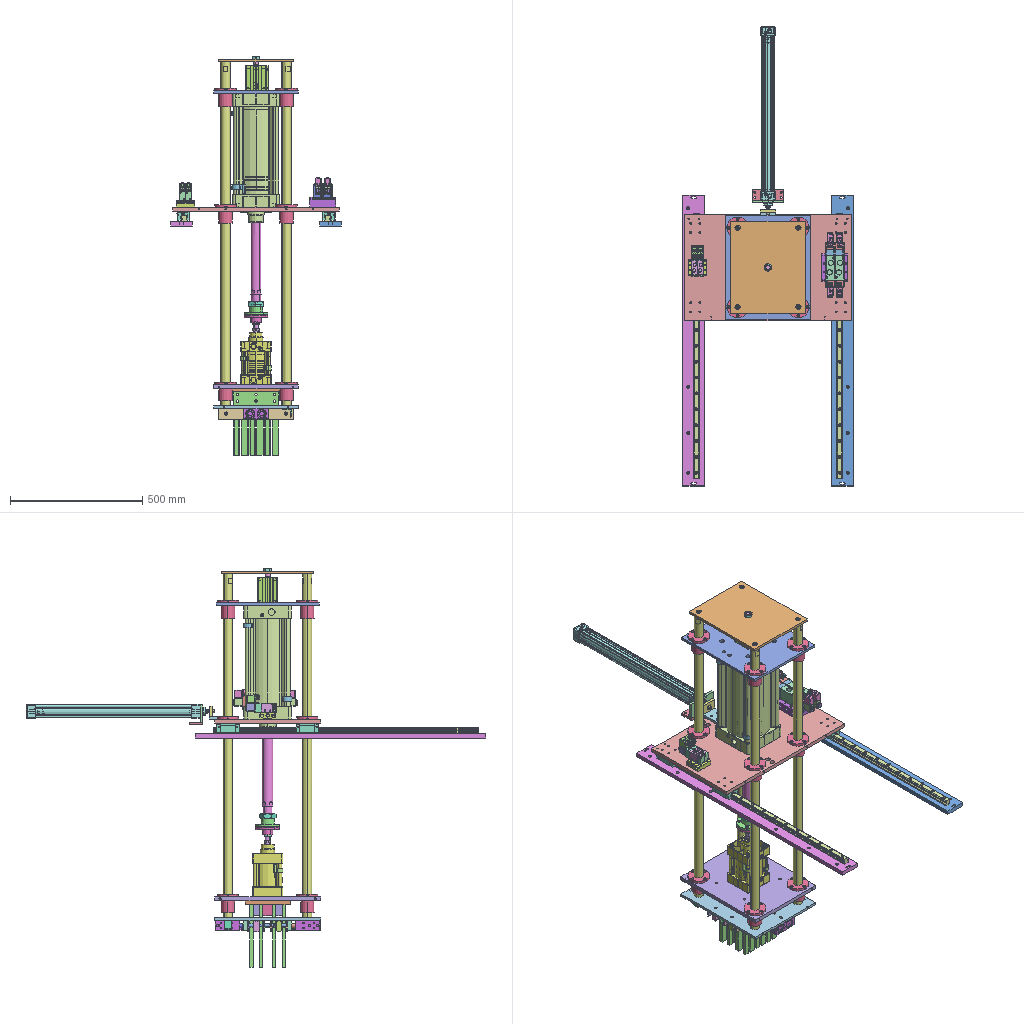Assembly | STEP file | 79 different items | 179 placed | box 643 x 1739 x 1508 mm
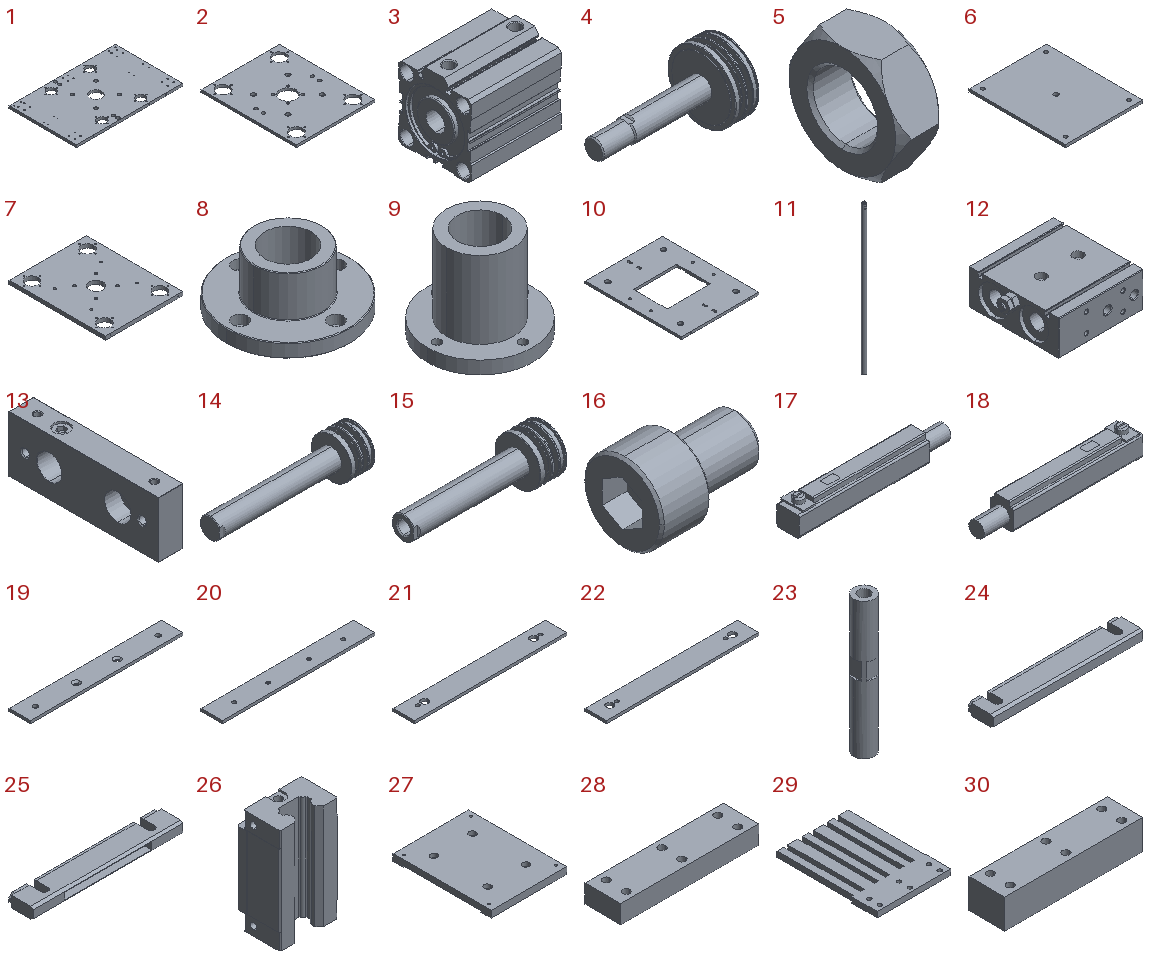Parts list (item | name | quantity | parent item | size | volume):
1 | 44-02-17 Press Cylinder Mounting Plate | x1 | in 44-01-00 Press-fit Slot Insertion Section2 | 630 x 400 x 15 mm | 3544491 mm3
2 | 44-02-18 Locating Cylinder Mounting Plate | x1 | in 44-01-00 Press-fit Slot Insertion Section2 | 320 x 390 x 10 mm | 1104020 mm3
3 | ACQS_63x50-1 | x1 | - | 96 x 77 x 84 mm | 270939 mm3
4 | ACQS_63x50-2 | x1 | - | 122 x 62.5 x 62.5 mm | 85364 mm3
5 | ACQS_63x50-3 | x1 | - | 11 x 31.177 x 27 mm | 4519 mm3
6 | 44-02-04 Locating Push Plate | x1 | in 44-01-00 Press-fit Slot Insertion Section2 | 280 x 350 x 10 mm | 972552 mm3
7 | 44-02-19 Press-fit Push Plate | x1 | in 44-01-00 Press-fit Slot Insertion Section2 | 320 x 400 x 15 mm | 1729546 mm3
8 | 44-02-20 Press Cylinder Connector | x1 | in 44-01-00 Press-fit Slot Insertion Section2 | 90 x 90 x 40 mm | 83101 mm3
9 | LHFRD35 | x12 | in 44-01-00 Press-fit Slot Insertion Section2 | 82 x 82 x 70 mm | 110033 mm3
10 | 44-02-21 Press-fit Locating Plate | x1 | in 44-01-00 Press-fit Slot Insertion Section2 | 320 x 400 x 10 mm | 995471 mm3
11 | 44-02-05 Press-fit Guide Shaft | x4 | in 44-01-00 Press-fit Slot Insertion Section2 | 35 x 35 x 1310 mm | 1250098 mm3
12 | TR_32x10-1 | x2 | - | 106 x 98 x 38 mm | 251208 mm3
13 | TR_32x10-2 | x2 | - | 16 x 96 x 36 mm | 48259 mm3
14 | TR_32x10-3 | x2 | - | 114.8 x 31.6 x 31.6 mm | 30621 mm3
15 | TR_32x10-4 | x2 | - | 98.8 x 31.6 x 31.6 mm | 26490 mm3
16 | TR_32x10-5 | x2 | - | 23.5 x 16 x 16 mm | 2769 mm3
17 | TR_32x10-6 | x2 | - | 30.5 x 4.4 x 5.5 mm | 552.742 mm3
18 | TR_32x10-7 | x2 | - | 30.5 x 4.4 x 5.5 mm | 552.742 mm3
19 | 44-02-06 Ear Forming Push Plate A | x1 | in 44-01-00 Press-fit Slot Insertion Section2 | 280 x 39 x 5 mm | 53413 mm3
20 | 44-02-07 Ear Forming Push Plate B | x1 | in 44-01-00 Press-fit Slot Insertion Section2 | 280 x 39 x 5 mm | 53633 mm3
21 | 44-02-08 Ear Forming Plate A | x1 | in 44-01-00 Press-fit Slot Insertion Section2 | 280 x 39 x 5 mm | 52910 mm3
22 | 44-02-09 Ear Forming Plate B | x1 | in 44-01-00 Press-fit Slot Insertion Section2 | 280 x 39 x 5 mm | 52910 mm3
23 | 44-02-10 Ear Forming Connecting Rod | x4 | in 44-01-00 Press-fit Slot Insertion Section2 | 12 x 12 x 81 mm | 7569 mm3
24 | 44-02-22 Ear Forming Locating Plate B | x1 | in 44-01-00 Press-fit Slot Insertion Section2 | 280 x 46 x 20.7 mm | 241213 mm3
25 | 44-02-23 Ear Forming Locating Plate C | x1 | in 44-01-00 Press-fit Slot Insertion Section2 | 280 x 46 x 20.7 mm | 145134 mm3
26 | HGH25CA | x4 | in 44-01-00 Press-fit Slot Insertion Section2 | 48 x 34.5 x 84 mm | 100839 mm3
27 | 44-02-013 Press-fit Fixing Plate | x1 | in 44-02-012 Press Plate Assembly | 170 x 220 x 15 mm | 464467 mm3
28 | 44-02-14 Press-fit Locating Plate | x2 | in 44-02-012 Press Plate Assembly | 173 x 45 x 23 mm | 168792 mm3
29 | 44-02-15 Press Plate | x4 | in 44-02-012 Press Plate Assembly | 173 x 240 x 13 mm | 402588 mm3
30 | 44-02-16 Press-fit Connecting Plate | x1 | in 44-02-012 Press Plate Assembly | 173 x 45 x 37 mm | 273922 mm3
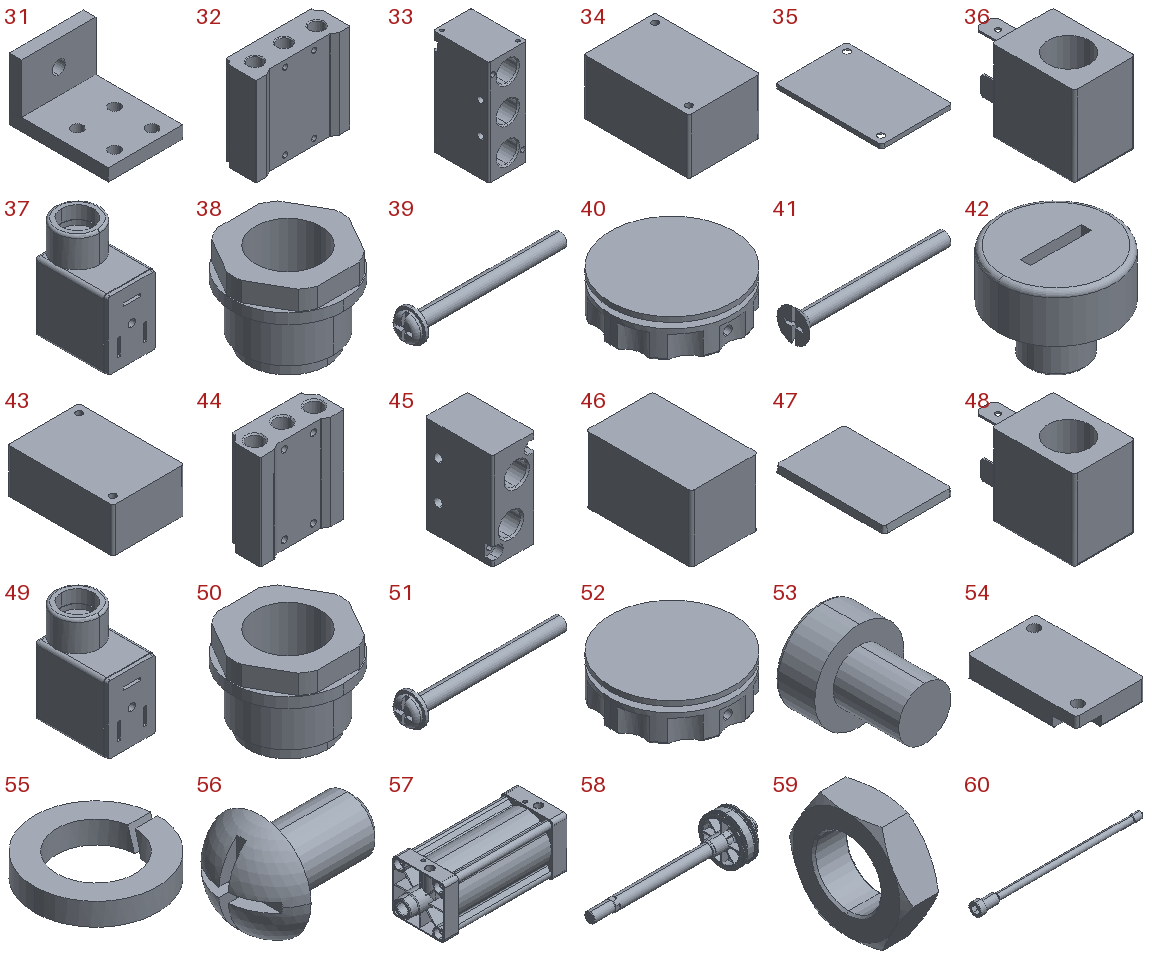31 | 44-02-011 Press Platform Push Plate | x1 | in 44-01-00 Press-fit Slot Insertion Section2 | 60 x 80 x 50 mm | 68539 mm3
32 | 400M_2F_400M-2F | x1 | in 44-01-00 Press-fit Slot Insertion Section2 | 104 x 38 x 98 mm | 289660 mm3
33 | 4V430C_15_Valve_Body | x2 | in 4V430C_15_B_4V430C-15-B | 34 x 50 x 94 mm | 133275 mm3
34 | 4V430C_15_Valve_Switch | x4 | in 4V430C_15_B_4V430C-15-B | 34 x 50 x 26.2 mm | 44112 mm3
35 | 4V430C_15_Valve_Board | x4 | in 4V430C_15_B_4V430C-15-B | 33.2 x 49.5 x 2 mm | 3202 mm3
36 | 4V430C_15_Valve_Coil | x4 | in 4V430C_15_B_4V430C-15-B | 22.3 x 44.2 x 30 mm | 14846 mm3
37 | 4V430C_15_Valve_Terminal | x4 | in 4V430C_15_B_4V430C-15-B | 21 x 32.2 x 41.5 mm | 20201 mm3
38 | 4V430C_15_Valve_Nut_T | x4 | in 4V430C_15_B_4V430C-15-B | 18.4 x 18.4 x 14 mm | 1443 mm3
39 | 4V430C_15_Valve_Bolt | x4 | in 4V430C_15_B_4V430C-15-B | 33.2 x 6.5 x 6.5 mm | 266.857 mm3
40 | 4V430C_15_Valve_Nut_C | x4 | in 4V430C_15_B_4V430C-15-B | 20 x 20 x 6.2 mm | 1695 mm3
41 | 4V430C_15_Valve_Screw_L | x8 | in 4V430C_15_B_4V430C-15-B | 32.2 x 7 x 6.954 mm | 247.49 mm3
42 | 4V430C_15_Valve_Button | x4 | in 4V430C_15_B_4V430C-15-B | 6.8 x 6.8 x 5.6 mm | 124.339 mm3
43 | 4V430C_15_Valve_Cover | x2 | in 4V430C_15_B_4V430C-15-B | 34 x 50 x 21 mm | 35377 mm3
44 | 200M_2F_200M-2F | x1 | in 44-01-00 Press-fit Slot Insertion Section2 | 61 x 26 x 69 mm | 73969 mm3
45 | - | x2 | in 4V210_08_B_4V210-08-B-P | 22 x 35 x 50 mm | 32799 mm3
46 | - | x2 | in 4V210_08_B_4V210-08-B-P | 22 x 35 x 22 mm | 16858 mm3
47 | - | x2 | in 4V210_08_B_4V210-08-B-P | 22 x 35 x 2.2 mm | 1664 mm3
48 | 4V200_Coil | x2 | in 4V210_08_B_4V210-08-B-P | 22.3 x 44.2 x 30 mm | 14846 mm3
49 | 4V200_Terminal | x2 | in 4V210_08_B_4V210-08-B-P | 21 x 32.2 x 41.5 mm | 20201 mm3
50 | 4V200_Terminal_Nut | x2 | in 4V210_08_B_4V210-08-B-P | 18.4 x 18.4 x 14 mm | 1443 mm3
51 | 4V200_Bolt | x2 | in 4V210_08_B_4V210-08-B-P | 33.2 x 6.5 x 6.5 mm | 266.857 mm3
52 | 4V200_Nut_C | x2 | in 4V210_08_B_4V210-08-B-P | 20 x 20 x 6.2 mm | 1695 mm3
53 | - | x2 | in 4V210_08_B_4V210-08-B-P | 6.8 x 8 x 6.8 mm | 164.101 mm3
54 | - | x2 | in 4V210_08_B_4V210-08-B-P | 22 x 35 x 6.7 mm | 4712 mm3
55 | - | x4 | in 4V210_08_B_4V210-08-B-P | 5.5 x 5.5 x 1 mm | 13.826 mm3
56 | - | x4 | in 4V210_08_B_4V210-08-B-P | 6.978 x 5.5 x 5.5 mm | 60.193 mm3
57 | - | x1 | - | 492 x 180 x 180 mm | 3117873 mm3
58 | - | x1 | - | 570 x 159 x 159 mm | 1181996 mm3
59 | - | x1 | - | 18 x 63.509 x 55 mm | 30482 mm3
60 | SI160_250 | x4 | - | 400 x 30 x 30 mm | 76937 mm3
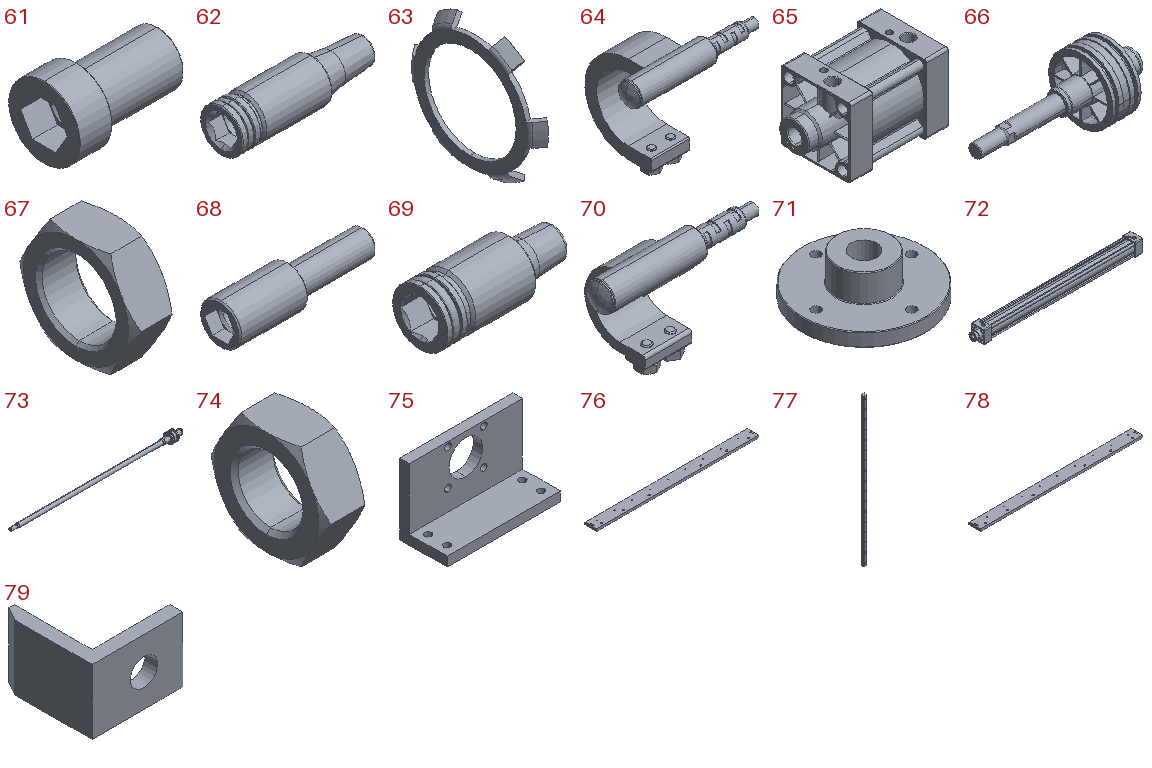61 | SI160 | x4 | - | 48 x 30 x 30 mm | 14480 mm3
62 | 160_C_Screw | x2 | - | 40 x 12 x 12 mm | 3167 mm3
63 | Outer_ring_gear_2 | x2 | - | 1.224 x 12 x 11.247 mm | 16.794 mm3
64 | CS1_B6 | x2 | - | 53.8 x 39.45 x 48.2 mm | 8992 mm3
65 | - | x1 | - | 203 x 115 x 115 mm | 819045 mm3
66 | - | x1 | - | 243 x 99 x 99 mm | 277761 mm3
67 | - | x1 | - | 10 x 30.022 x 26 mm | 3125 mm3
68 | SI100_25 | x8 | - | 55 x 15.5 x 15.5 mm | 5807 mm3
69 | 100_C_Screw | x2 | - | 24.2 x 10 x 10 mm | 1321 mm3
70 | CS1_B4 | x2 | - | 53.8 x 25.85 x 38.4 mm | 5585 mm3
71 | 44-02-24 Press Cylinder Connector | x1 | in 44-01-00 Press-fit Slot Insertion Section2 | 90 x 90 x 30 mm | 79238 mm3
72 | SI_40x550-1 | x1 | - | 679.5 x 53 x 53 mm | 489636 mm3
73 | SI_40x550-2 | x1 | - | 695.5 x 39.5 x 39.5 mm | 154171 mm3
74 | SI_40x550-3 | x1 | - | 7 x 19.63 x 17 mm | 1102 mm3
75 | 44-02-03 Cylinder Mounting Kit | x1 | in 44-01-00 Press-fit Slot Insertion Section2 | 120 x 50 x 75 mm | 124742 mm3
76 | 44-02-01 Guide Rail Mounting Plate A | x1 | in 44-01-00 Press-fit Slot Insertion Section2 | 1100 x 80 x 16 mm | 1395246 mm3
77 | HGH 25HA-950 | x2 | in 44-01-00 Press-fit Slot Insertion Section2 | 23 x 22 x 1000 mm | 420521 mm3
78 | 44-02-02 Guide Rail Mounting Plate B | x1 | in 44-01-00 Press-fit Slot Insertion Section2 | 1100 x 80 x 16 mm | 1395246 mm3
79 | 44-02-25 Lower Ejector Guide Plate | x2 | in 44-01-00 Press-fit Slot Insertion Section2 | 35 x 35 x 25 mm | 7497 mm3
Placements (level | parent | child | x y z in mm | rotation matrix by rows):
1 | 44-01-00 Press-fit Slot Insertion Section2 | 44-02-17 Press Cylinder Mounting Plate | -20.096 -11.932 -0.0 | 1 0 0 0 1 0 0 0 1
1 | 44-01-00 Press-fit Slot Insertion Section2 | 44-02-18 Locating Cylinder Mounting Plate | -20.096 -11.932 437.5 | 1 0 0 0 1 0 0 0 1
1 | 44-01-00 Press-fit Slot Insertion Section2 | subassembly 2 | -20.096 -11.932 543.5 | 0 0 1 0 1 0 -1 0 0
2 | subassembly 2 | ACQS_63x50-1 | -0.0 -0.0 -0.0 | 1 0 0 0 1 0 0 0 1
2 | subassembly 2 | ACQS_63x50-2 | -0.0 -0.0 -0.0 | 1 0 0 0 0.2744 0.9616 0 -0.9616 0.2744
2 | subassembly 2 | ACQS_63x50-3 | -7.5 0.0 -0.0 | 1 0 0 0 0.9981 0.06174 0 -0.06174 0.9981
1 | 44-01-00 Press-fit Slot Insertion Section2 | 44-02-04 Locating Push Plate | -20.096 -11.932 557.5 | -1 0 0 0 -1 0 0 0 1
1 | 44-01-00 Press-fit Slot Insertion Section2 | 44-02-19 Press-fit Push Plate | -20.096 -11.932 -671.0 | 1 0 0 0 1 0 0 0 1
1 | 44-01-00 Press-fit Slot Insertion Section2 | 44-02-20 Press Cylinder Connector | -20.096 -11.932 -399.5 | -0.6148 -0.7887 0 0.7887 -0.6148 0 0 0 1
1 | 44-01-00 Press-fit Slot Insertion Section2 | LHFRD35 | -135.096 138.068 457.5 | -1 0 0 0 1 0 0 0 -1
1 | 44-01-00 Press-fit Slot Insertion Section2 | LHFRD35 | -135.096 -161.932 457.5 | -1 0 0 0 1 0 0 0 -1
1 | 44-01-00 Press-fit Slot Insertion Section2 | LHFRD35 | 94.903 -161.932 457.5 | -1 0 0 0 1 0 0 0 -1
1 | 44-01-00 Press-fit Slot Insertion Section2 | LHFRD35 | 94.903 138.068 457.5 | -1 0 0 0 1 0 0 0 -1
1 | 44-01-00 Press-fit Slot Insertion Section2 | LHFRD35 | 94.903 138.068 17.5 | -1 0 0 0 1 0 0 0 -1
1 | 44-01-00 Press-fit Slot Insertion Section2 | LHFRD35 | 94.903 -161.932 17.5 | -1 0 0 0 1 0 0 0 -1
1 | 44-01-00 Press-fit Slot Insertion Section2 | LHFRD35 | -135.096 138.068 17.5 | -1 0 0 0 1 0 0 0 -1
1 | 44-01-00 Press-fit Slot Insertion Section2 | LHFRD35 | -135.096 -161.932 17.5 | -1 0 0 0 1 0 0 0 -1
1 | 44-01-00 Press-fit Slot Insertion Section2 | LHFRD35 | 94.903 -161.932 -653.5 | -1 0 0 0 1 0 0 0 -1
1 | 44-01-00 Press-fit Slot Insertion Section2 | LHFRD35 | 94.903 138.068 -653.5 | -1 0 0 0 1 0 0 0 -1
1 | 44-01-00 Press-fit Slot Insertion Section2 | LHFRD35 | -135.096 -161.932 -653.5 | -1 0 0 0 1 0 0 0 -1
1 | 44-01-00 Press-fit Slot Insertion Section2 | LHFRD35 | -135.096 138.068 -653.5 | -1 0 0 0 1 0 0 0 -1
1 | 44-01-00 Press-fit Slot Insertion Section2 | 44-02-21 Press-fit Locating Plate | -20.096 -11.932 -748.5 | 1 0 0 0 1 0 0 0 1
1 | 44-01-00 Press-fit Slot Insertion Section2 | 44-02-05 Press-fit Guide Shaft | -135.096 138.068 -88.5 | -0.5385 -0.8426 0 0.8426 -0.5385 0 0 0 1
1 | 44-01-00 Press-fit Slot Insertion Section2 | 44-02-05 Press-fit Guide Shaft | 94.903 138.068 -88.5 | 1 0 0 0 1 0 0 0 1
1 | 44-01-00 Press-fit Slot Insertion Section2 | 44-02-05 Press-fit Guide Shaft | 94.903 -161.932 -88.5 | 0.9008 -0.4343 0 0.4343 0.9008 0 0 0 1
1 | 44-01-00 Press-fit Slot Insertion Section2 | 44-02-05 Press-fit Guide Shaft | -135.096 -161.932 -88.5 | 1 0 0 0 1 0 0 0 1
1 | 44-01-00 Press-fit Slot Insertion Section2 | subassembly 3 | -20.096 -117.932 -753.5 | 0 -1 0 -1 0 0 0 0 -1
2 | subassembly 3 | TR_32x10-1 | -0.0 -0.0 -0.0 | 1 0 0 0 1 0 0 0 1
2 | subassembly 3 | TR_32x10-2 | -0.0 -0.0 -0.0 | 1 0 0 0 1 0 0 0 1
2 | subassembly 3 | TR_32x10-3 | -0.0 -0.0 -0.0 | 1 0 0 0 1 0 0 0 1
2 | subassembly 3 | TR_32x10-4 | -0.0 -0.0 -0.0 | 1 0 0 0 1 0 0 0 1
2 | subassembly 3 | TR_32x10-5 | -0.0 -0.0 -0.0 | 1 0 0 0 1 0 0 0 1
2 | subassembly 3 | TR_32x10-6 | -0.0 -0.0 -0.0 | 1 0 0 0 1 0 0 0 1
2 | subassembly 3 | TR_32x10-7 | -0.0 -0.0 -0.0 | 1 0 0 0 1 0 0 0 1
1 | 44-01-00 Press-fit Slot Insertion Section2 | subassembly 3 | -20.096 94.068 -753.5 | 0 1 0 1 0 0 0 0 -1
2 | subassembly 3 | TR_32x10-1 | -0.0 -0.0 -0.0 | 1 0 0 0 1 0 0 0 1
2 | subassembly 3 | TR_32x10-2 | -0.0 -0.0 -0.0 | 1 0 0 0 1 0 0 0 1
2 | subassembly 3 | TR_32x10-3 | -0.0 -0.0 -0.0 | 1 0 0 0 1 0 0 0 1
2 | subassembly 3 | TR_32x10-4 | -0.0 -0.0 -0.0 | 1 0 0 0 1 0 0 0 1
2 | subassembly 3 | TR_32x10-5 | -0.0 -0.0 -0.0 | 1 0 0 0 1 0 0 0 1
2 | subassembly 3 | TR_32x10-6 | -0.0 -0.0 -0.0 | 1 0 0 0 1 0 0 0 1
2 | subassembly 3 | TR_32x10-7 | -0.0 -0.0 -0.0 | 1 0 0 0 1 0 0 0 1
1 | 44-01-00 Press-fit Slot Insertion Section2 | 44-02-06 Ear Forming Push Plate A | -20.096 -85.432 -772.5 | 1 0 0 0 0 1 0 -1 -0
1 | 44-01-00 Press-fit Slot Insertion Section2 | 44-02-07 Ear Forming Push Plate B | -20.096 61.568 -772.5 | 1 0 0 0 0 1 0 -1 -0
1 | 44-01-00 Press-fit Slot Insertion Section2 | 44-02-08 Ear Forming Plate A | -20.096 0.5677 -772.5 | 1 0 0 0 0 -1 0 1 0
1 | 44-01-00 Press-fit Slot Insertion Section2 | 44-02-09 Ear Forming Plate B | -20.096 -24.432 -772.5 | 1 0 0 0 0 -1 0 1 0
1 | 44-01-00 Press-fit Slot Insertion Section2 | 44-02-10 Ear Forming Connecting Rod | 92.403 -42.432 -772.5 | -0.8372 -0.5469 0 0 0 1 -0.5469 0.8372 -0
1 | 44-01-00 Press-fit Slot Insertion Section2 | 44-02-10 Ear Forming Connecting Rod | -132.596 -42.432 -772.5 | -0.8372 -0.5469 0 0 0 1 -0.5469 0.8372 -0
1 | 44-01-00 Press-fit Slot Insertion Section2 | 44-02-10 Ear Forming Connecting Rod | 79.903 18.568 -772.5 | 1 0 0 0 0 -1 0 1 0
1 | 44-01-00 Press-fit Slot Insertion Section2 | 44-02-10 Ear Forming Connecting Rod | -120.097 18.568 -772.5 | -0.0524 0.9986 0 0 0 -1 -0.9986 -0.0524 0
1 | 44-01-00 Press-fit Slot Insertion Section2 | 44-02-22 Ear Forming Locating Plate B | -20.096 -54.932 -773.5 | 1 0 0 0 0 -1 0 1 0
1 | 44-01-00 Press-fit Slot Insertion Section2 | 44-02-23 Ear Forming Locating Plate C | -20.096 31.068 -773.5 | 1 0 0 0 0 -1 0 1 0
1 | 44-01-00 Press-fit Slot Insertion Section2 | HGH25CA | 254.904 138.068 -47.5 | 1 0 0 0 0 -1 0 1 0
1 | 44-01-00 Press-fit Slot Insertion Section2 | HGH25CA | 254.904 -161.932 -47.5 | 1 0 0 0 0 -1 0 1 0
1 | 44-01-00 Press-fit Slot Insertion Section2 | HGH25CA | -295.096 138.068 -47.5 | 1 0 0 0 0 -1 0 1 0
1 | 44-01-00 Press-fit Slot Insertion Section2 | HGH25CA | -295.096 -161.932 -47.5 | 1 0 0 0 0 -1 0 1 0
1 | 44-01-00 Press-fit Slot Insertion Section2 | 44-02-012 Press Plate Assembly | -47.286 -33.384 -686.0 | 0 1 0 -1 0 0 0 0 1
2 | 44-02-012 Press Plate Assembly | 44-02-013 Press-fit Fixing Plate | -21.452 27.189 -0.0 | 1 0 0 0 1 0 0 0 1
2 | 44-02-012 Press Plate Assembly | 44-02-14 Press-fit Locating Plate | -64.452 27.189 -27.0 | 0 0 1 1 0 0 0 1 0
2 | 44-02-012 Press Plate Assembly | 44-02-14 Press-fit Locating Plate | 21.548 27.189 -27.0 | 0 0 1 1 0 0 0 1 0
2 | 44-02-012 Press Plate Assembly | 44-02-15 Press Plate | -82.452 27.189 -124.5 | 0 0 1 -1 0 0 0 -1 0
2 | 44-02-012 Press Plate Assembly | 44-02-15 Press Plate | -46.452 27.189 -124.5 | 0 0 -1 1 0 0 0 -1 0
2 | 44-02-012 Press Plate Assembly | 44-02-15 Press Plate | 3.548 27.189 -124.5 | 0 0 1 -1 0 0 0 -1 0
2 | 44-02-012 Press Plate Assembly | 44-02-15 Press Plate | 39.548 27.189 -124.5 | 0 0 -1 1 0 0 0 -1 0
2 | 44-02-012 Press Plate Assembly | 44-02-16 Press-fit Connecting Plate | -21.452 27.189 -27.0 | 0 0 -1 -1 0 0 0 1 0
1 | 44-01-00 Press-fit Slot Insertion Section2 | 44-02-011 Press Platform Push Plate | -20.096 168.068 12.5 | 1 0 0 0 1 0 0 0 1
1 | 44-01-00 Press-fit Slot Insertion Section2 | 400M_2F_400M-2F | 183.904 -11.932 7.5 | 0 0 1 1 0 0 0 1 0
1 | 44-01-00 Press-fit Slot Insertion Section2 | 4V430C_15_B_4V430C-15-B | 215.404 -58.932 70.5 | 1 0 0 0 0 -1 0 1 0
2 | 4V430C_15_B_4V430C-15-B | 4V430C_15_Valve_Body | -0.0 -0.0 -0.0 | 1 0 0 0 1 0 0 0 1
2 | 4V430C_15_B_4V430C-15-B | 4V430C_15_Valve_Switch | -0.0 -0.0 -0.0 | -1 0 0 0 1 0 0 0 -1
2 | 4V430C_15_B_4V430C-15-B | 4V430C_15_Valve_Board | -0.0 -0.0 26.2 | -1 0 0 0 1 0 0 0 -1
2 | 4V430C_15_B_4V430C-15-B | 4V430C_15_Valve_Coil | -0.0 -0.0 28.2 | -1 0 0 0 1 0 0 0 -1
2 | 4V430C_15_B_4V430C-15-B | 4V430C_15_Valve_Terminal | -0.0 -0.0 28.2 | -1 0 0 0 1 0 0 0 -1
2 | 4V430C_15_B_4V430C-15-B | 4V430C_15_Valve_Nut_T | -0.0 -0.0 28.2 | -1 0 0 0 1 0 0 0 -1
2 | 4V430C_15_B_4V430C-15-B | 4V430C_15_Valve_Bolt | -0.0 46.7 43.2 | 0 0 1 -1 0 0 0 -1 0
2 | 4V430C_15_B_4V430C-15-B | 4V430C_15_Valve_Nut_C | -0.0 -0.0 28.2 | -1 0 0 0 1 0 0 0 -1
2 | 4V430C_15_B_4V430C-15-B | 4V430C_15_Valve_Screw_L | -13.0 21.0 28.2 | 0 0 1 0 1 0 -1 0 0
2 | 4V430C_15_B_4V430C-15-B | 4V430C_15_Valve_Screw_L | 13.0 -21.0 28.2 | 0 0 1 0 1 0 -1 0 0
2 | 4V430C_15_B_4V430C-15-B | 4V430C_15_Valve_Button | 0.0 25.0 17.6 | -1 0 0 0 0 1 0 1 0
2 | 4V430C_15_B_4V430C-15-B | 4V430C_15_Valve_Cover | -0.0 -0.0 -94.0 | 1 0 0 0 1 0 0 0 1
2 | 4V430C_15_B_4V430C-15-B | 4V430C_15_Valve_Switch | -0.0 -0.0 -115.0 | 1 0 0 0 1 0 0 0 1
2 | 4V430C_15_B_4V430C-15-B | 4V430C_15_Valve_Board | -0.0 -0.0 -141.2 | 1 0 0 0 1 0 0 0 1
2 | 4V430C_15_B_4V430C-15-B | 4V430C_15_Valve_Coil | -0.0 -0.0 -143.2 | 1 0 0 0 1 0 0 0 1
2 | 4V430C_15_B_4V430C-15-B | 4V430C_15_Valve_Terminal | -0.0 -0.0 -143.2 | 1 0 0 0 1 0 0 0 1
2 | 4V430C_15_B_4V430C-15-B | 4V430C_15_Valve_Nut_T | -0.0 -0.0 -143.2 | 1 0 0 0 1 0 0 0 1
2 | 4V430C_15_B_4V430C-15-B | 4V430C_15_Valve_Bolt | -0.0 46.7 -158.2 | 0 0 -1 -1 0 0 0 1 0
2 | 4V430C_15_B_4V430C-15-B | 4V430C_15_Valve_Nut_C | -0.0 -0.0 -143.2 | 1 0 0 0 1 0 0 0 1
2 | 4V430C_15_B_4V430C-15-B | 4V430C_15_Valve_Screw_L | 13.0 21.0 -143.2 | 0 0 -1 0 1 0 1 0 0
2 | 4V430C_15_B_4V430C-15-B | 4V430C_15_Valve_Screw_L | -13.0 -21.0 -143.2 | 0 0 -1 0 1 0 1 0 0
2 | 4V430C_15_B_4V430C-15-B | 4V430C_15_Valve_Button | -0.0 25.0 -132.6 | 1 0 0 0 0 1 0 -1 0
1 | 44-01-00 Press-fit Slot Insertion Section2 | 4V430C_15_B_4V430C-15-B | 250.404 -58.932 70.5 | 1 0 0 0 0 -1 0 1 0
2 | 4V430C_15_B_4V430C-15-B | 4V430C_15_Valve_Body | -0.0 -0.0 -0.0 | 1 0 0 0 1 0 0 0 1
2 | 4V430C_15_B_4V430C-15-B | 4V430C_15_Valve_Switch | -0.0 -0.0 -0.0 | -1 0 0 0 1 0 0 0 -1
2 | 4V430C_15_B_4V430C-15-B | 4V430C_15_Valve_Board | -0.0 -0.0 26.2 | -1 0 0 0 1 0 0 0 -1
2 | 4V430C_15_B_4V430C-15-B | 4V430C_15_Valve_Coil | -0.0 -0.0 28.2 | -1 0 0 0 1 0 0 0 -1
2 | 4V430C_15_B_4V430C-15-B | 4V430C_15_Valve_Terminal | -0.0 -0.0 28.2 | -1 0 0 0 1 0 0 0 -1
2 | 4V430C_15_B_4V430C-15-B | 4V430C_15_Valve_Nut_T | -0.0 -0.0 28.2 | -1 0 0 0 1 0 0 0 -1
2 | 4V430C_15_B_4V430C-15-B | 4V430C_15_Valve_Bolt | -0.0 46.7 43.2 | 0 0 1 -1 0 0 0 -1 0
2 | 4V430C_15_B_4V430C-15-B | 4V430C_15_Valve_Nut_C | -0.0 -0.0 28.2 | -1 0 0 0 1 0 0 0 -1
2 | 4V430C_15_B_4V430C-15-B | 4V430C_15_Valve_Screw_L | -13.0 21.0 28.2 | 0 0 1 0 1 0 -1 0 0
2 | 4V430C_15_B_4V430C-15-B | 4V430C_15_Valve_Screw_L | 13.0 -21.0 28.2 | 0 0 1 0 1 0 -1 0 0
2 | 4V430C_15_B_4V430C-15-B | 4V430C_15_Valve_Button | 0.0 25.0 17.6 | -1 0 0 0 0 1 0 1 0
2 | 4V430C_15_B_4V430C-15-B | 4V430C_15_Valve_Cover | -0.0 -0.0 -94.0 | 1 0 0 0 1 0 0 0 1
2 | 4V430C_15_B_4V430C-15-B | 4V430C_15_Valve_Switch | -0.0 -0.0 -115.0 | 1 0 0 0 1 0 0 0 1
2 | 4V430C_15_B_4V430C-15-B | 4V430C_15_Valve_Board | -0.0 -0.0 -141.2 | 1 0 0 0 1 0 0 0 1
2 | 4V430C_15_B_4V430C-15-B | 4V430C_15_Valve_Coil | -0.0 -0.0 -143.2 | 1 0 0 0 1 0 0 0 1
2 | 4V430C_15_B_4V430C-15-B | 4V430C_15_Valve_Terminal | -0.0 -0.0 -143.2 | 1 0 0 0 1 0 0 0 1
2 | 4V430C_15_B_4V430C-15-B | 4V430C_15_Valve_Nut_T | -0.0 -0.0 -143.2 | 1 0 0 0 1 0 0 0 1
2 | 4V430C_15_B_4V430C-15-B | 4V430C_15_Valve_Bolt | -0.0 46.7 -158.2 | 0 0 -1 -1 0 0 0 1 0
2 | 4V430C_15_B_4V430C-15-B | 4V430C_15_Valve_Nut_C | -0.0 -0.0 -143.2 | 1 0 0 0 1 0 0 0 1
2 | 4V430C_15_B_4V430C-15-B | 4V430C_15_Valve_Screw_L | 13.0 21.0 -143.2 | 0 0 -1 0 1 0 1 0 0
2 | 4V430C_15_B_4V430C-15-B | 4V430C_15_Valve_Screw_L | -13.0 -21.0 -143.2 | 0 0 -1 0 1 0 1 0 0
2 | 4V430C_15_B_4V430C-15-B | 4V430C_15_Valve_Button | -0.0 25.0 -132.6 | 1 0 0 0 0 1 0 -1 0
1 | 44-01-00 Press-fit Slot Insertion Section2 | 200M_2F_200M-2F | -252.096 -11.932 7.5 | 0 0 -1 -1 0 0 0 1 0
1 | 44-01-00 Press-fit Slot Insertion Section2 | 4V210_08_B_4V210-08-B-P | -298.096 -11.932 51.0 | 1 0 0 0 0 -1 0 1 0
2 | 4V210_08_B_4V210-08-B-P | subassembly 4 | -0.0 -0.0 -25.0 | -1 0 0 0 -1 0 0 0 1
2 | 4V210_08_B_4V210-08-B-P | subassembly 5 | -0.0 -0.0 -25.0 | -1 0 0 0 1 0 0 0 -1
2 | 4V210_08_B_4V210-08-B-P | subassembly 6 | -0.0 -0.0 -47.0 | -1 0 0 0 1 0 0 0 -1
2 | 4V210_08_B_4V210-08-B-P | 4V200_Coil | -0.0 -0.0 -49.2 | 1 0 0 0 1 0 0 0 1
2 | 4V210_08_B_4V210-08-B-P | 4V200_Terminal | -0.0 -0.0 -49.2 | 1 0 0 0 1 0 0 0 1
2 | 4V210_08_B_4V210-08-B-P | 4V200_Terminal_Nut | -0.0 -0.0 -49.2 | 1 0 0 0 1 0 0 0 1
2 | 4V210_08_B_4V210-08-B-P | 4V200_Bolt | -0.0 46.7 -64.2 | 0 0 -1 -1 0 0 0 1 0
2 | 4V210_08_B_4V210-08-B-P | 4V200_Nut_C | -0.0 -0.0 -49.2 | 0 1 0 -1 0 0 0 0 1
2 | 4V210_08_B_4V210-08-B-P | subassembly 7 | 0.0 12.5 -38.3 | 0 0 1 0 1 0 -1 0 0
2 | 4V210_08_B_4V210-08-B-P | subassembly 8 | -0.0 -0.0 31.7 | 1 0 0 0 -1 0 0 0 -1
2 | 4V210_08_B_4V210-08-B-P | subassembly 9 | 7.0 -14.0 28.4 | 1 0 0 0 1 0 0 0 1
2 | 4V210_08_B_4V210-08-B-P | subassembly 10 | 7.0 -14.0 29.4 | 0 0 -1 0 -1 0 -1 0 0
2 | 4V210_08_B_4V210-08-B-P | subassembly 9 | -7.0 14.0 28.4 | 1 0 0 0 1 0 0 0 1
2 | 4V210_08_B_4V210-08-B-P | subassembly 10 | -7.0 14.0 29.4 | 0 0 -1 0 -1 0 -1 0 0
1 | 44-01-00 Press-fit Slot Insertion Section2 | 4V210_08_B_4V210-08-B-P | -275.096 -11.932 51.0 | 1 0 0 0 0 -1 0 1 0
2 | 4V210_08_B_4V210-08-B-P | subassembly 4 | -0.0 -0.0 -25.0 | -1 0 0 0 -1 0 0 0 1
2 | 4V210_08_B_4V210-08-B-P | subassembly 5 | -0.0 -0.0 -25.0 | -1 0 0 0 1 0 0 0 -1
2 | 4V210_08_B_4V210-08-B-P | subassembly 6 | -0.0 -0.0 -47.0 | -1 0 0 0 1 0 0 0 -1
2 | 4V210_08_B_4V210-08-B-P | 4V200_Coil | -0.0 -0.0 -49.2 | 1 0 0 0 1 0 0 0 1
2 | 4V210_08_B_4V210-08-B-P | 4V200_Terminal | -0.0 -0.0 -49.2 | 1 0 0 0 1 0 0 0 1
2 | 4V210_08_B_4V210-08-B-P | 4V200_Terminal_Nut | -0.0 -0.0 -49.2 | 1 0 0 0 1 0 0 0 1
2 | 4V210_08_B_4V210-08-B-P | 4V200_Bolt | -0.0 46.7 -64.2 | 0 0 -1 -1 0 0 0 1 0
2 | 4V210_08_B_4V210-08-B-P | 4V200_Nut_C | -0.0 -0.0 -49.2 | 0 1 0 -1 0 0 0 0 1
2 | 4V210_08_B_4V210-08-B-P | subassembly 7 | 0.0 12.5 -38.3 | 0 0 1 0 1 0 -1 0 0
2 | 4V210_08_B_4V210-08-B-P | subassembly 8 | -0.0 -0.0 31.7 | 1 0 0 0 -1 0 0 0 -1
2 | 4V210_08_B_4V210-08-B-P | subassembly 9 | 7.0 -14.0 28.4 | 1 0 0 0 1 0 0 0 1
2 | 4V210_08_B_4V210-08-B-P | subassembly 10 | 7.0 -14.0 29.4 | 0 0 -1 0 -1 0 -1 0 0
2 | 4V210_08_B_4V210-08-B-P | subassembly 9 | -7.0 14.0 28.4 | 1 0 0 0 1 0 0 0 1
2 | 4V210_08_B_4V210-08-B-P | subassembly 10 | -7.0 14.0 29.4 | 0 0 -1 0 -1 0 -1 0 0
1 | 44-01-00 Press-fit Slot Insertion Section2 | subassembly 11 | -20.096 -11.932 7.5 | 0 0 -1 0 1 0 1 0 0
2 | subassembly 11 | subassembly 12 | -0.0 -0.0 -0.0 | 1 0 0 0 1 0 0 0 1
2 | subassembly 11 | subassembly 13 | -250.0 -0.0 -0.0 | 1 0 0 0 0.7071 0.7071 0 -0.7071 0.7071
2 | subassembly 11 | subassembly 14 | -375.0 0.0 0.0 | 1 0 0 0 -1 0 0 0 -1
2 | subassembly 11 | SI160_250 | 50.0 -70.0 70.0 | 1 0 0 0 1 0 0 0 1
2 | subassembly 11 | SI160_250 | 50.0 -70.0 -70.0 | 1 0 0 0 1 0 0 0 1
2 | subassembly 11 | SI160_250 | 50.0 70.0 70.0 | 1 0 0 0 1 0 0 0 1
2 | subassembly 11 | SI160_250 | 50.0 70.0 -70.0 | 1 0 0 0 1 0 0 0 1
2 | subassembly 11 | SI160 | 380.0 -70.0 70.0 | -1 0 0 0 -1 0 0 0 1
2 | subassembly 11 | SI160 | 380.0 -70.0 -70.0 | -1 0 0 0 -1 0 0 0 1
2 | subassembly 11 | SI160 | 380.0 70.0 70.0 | -1 0 0 0 -1 0 0 0 1
2 | subassembly 11 | SI160 | 380.0 70.0 -70.0 | -1 0 0 0 -1 0 0 0 1
2 | subassembly 11 | 160_C_Screw | 37.0 20.0 86.5 | 0 0 -1 0 -1 0 -1 0 0
2 | subassembly 11 | 160_C_Screw | 393.0 20.0 86.5 | 0 0 -1 0 -1 0 -1 0 0
2 | subassembly 11 | Outer_ring_gear_2 | 37.0 20.0 88.7 | 0 -1 0 0 0 -1 1 0 0
2 | subassembly 11 | Outer_ring_gear_2 | 393.0 20.0 88.7 | 0 -1 0 0 0 -1 1 0 0
2 | subassembly 11 | CS1_B6 | 52.8 -72.832 72.832 | 1 0 0 0 -0.7193 -0.6947 0 0.6947 -0.7193
2 | subassembly 11 | CS1_B6 | 377.2 72.832 72.832 | -1 0 0 0 0.7193 0.6947 0 0.6947 -0.7193
1 | 44-01-00 Press-fit Slot Insertion Section2 | subassembly 15 | -20.096 -11.932 -500.5 | 0 1 0 0 0 -1 -1 0 0
2 | subassembly 15 | subassembly 16 | -0.0 -0.0 -0.0 | 1 0 0 0 1 0 0 0 1
2 | subassembly 15 | subassembly 17 | -0.0 -0.0 -0.0 | 1 0 0 0 0.7071 0.7071 0 -0.7071 0.7071
2 | subassembly 15 | subassembly 18 | -76.0 -0.0 0.0 | 1 0 0 0 -1 0 0 0 -1
2 | subassembly 15 | SI100_25 | 27.0 -44.5 44.5 | 1 0 0 0 1 0 0 0 1
2 | subassembly 15 | SI100_25 | 27.0 -44.5 -44.5 | 1 0 0 0 1 0 0 0 1
2 | subassembly 15 | SI100_25 | 27.0 44.5 44.5 | 1 0 0 0 1 0 0 0 1
2 | subassembly 15 | SI100_25 | 27.0 44.5 -44.5 | 1 0 0 0 1 0 0 0 1
2 | subassembly 15 | SI100_25 | 136.0 -44.5 44.5 | -1 0 0 0 -1 0 0 0 1
2 | subassembly 15 | SI100_25 | 136.0 -44.5 -44.5 | -1 0 0 0 -1 0 0 0 1
2 | subassembly 15 | SI100_25 | 136.0 44.5 44.5 | -1 0 0 0 -1 0 0 0 1
2 | subassembly 15 | SI100_25 | 136.0 44.5 -44.5 | -1 0 0 0 -1 0 0 0 1
2 | subassembly 15 | 100_C_Screw | 27.0 13.5 55.0 | 0 0 -1 0 -1 0 -1 0 0
2 | subassembly 15 | 100_C_Screw | 136.0 13.5 55.0 | 0 0 -1 0 -1 0 -1 0 0
2 | subassembly 15 | CS1_B4 | 39.8 -45.997 45.997 | 1 0 0 0 -0.7193 -0.6947 0 0.6947 -0.7193
2 | subassembly 15 | CS1_B4 | 123.2 45.997 45.997 | -1 0 0 0 0.7193 0.6947 0 0.6947 -0.7193
1 | 44-01-00 Press-fit Slot Insertion Section2 | 44-02-24 Press Cylinder Connector | -20.096 -11.932 -399.5 | 0.7887 0.6148 0 0.6148 -0.7887 0 0 0 -1
1 | 44-01-00 Press-fit Slot Insertion Section2 | subassembly 19 | 61.906 322.226 -85.305 | 0 -1 0 1 0 0 0 0 1
2 | subassembly 19 | SI_40x550-1 | -79.158 82.003 122.805 | 1 0 0 0 1 0 0 0 1
2 | subassembly 19 | SI_40x550-2 | -79.158 82.003 122.805 | 1 0 0 0 -0.01178 -0.9999 0 0.9999 -0.01178
2 | subassembly 19 | SI_40x550-3 | -79.158 82.003 122.805 | 1 0 0 0 -0.7055 -0.7087 0 0.7087 -0.7055
1 | 44-01-00 Press-fit Slot Insertion Section2 | 44-02-03 Cylinder Mounting Kit | -20.096 258.068 -8.5 | -1 0 0 0 -1 0 0 0 1
1 | 44-01-00 Press-fit Slot Insertion Section2 | 44-02-01 Guide Rail Mounting Plate A | 261.454 -287.432 -55.5 | 0 -1 0 1 0 0 0 0 1
1 | 44-01-00 Press-fit Slot Insertion Section2 | HGH 25HA-950 | 251.453 -399.932 -47.5 | 1 0 0 0 0 -1 0 1 -0
1 | 44-01-00 Press-fit Slot Insertion Section2 | 44-02-02 Guide Rail Mounting Plate B | -301.647 -287.432 -55.5 | 0 1 0 -1 0 0 0 0 1
1 | 44-01-00 Press-fit Slot Insertion Section2 | HGH 25HA-950 | -291.647 -399.932 -47.5 | 1 0 0 0 0 -1 0 1 0
1 | 44-01-00 Press-fit Slot Insertion Section2 | 44-02-25 Lower Ejector Guide Plate | -155.096 138.068 -753.5 | 1 0 0 0 0 1 0 -1 0
1 | 44-01-00 Press-fit Slot Insertion Section2 | 44-02-25 Lower Ejector Guide Plate | 114.903 -161.932 -753.5 | -1 0 0 0 0 -1 0 -1 -0